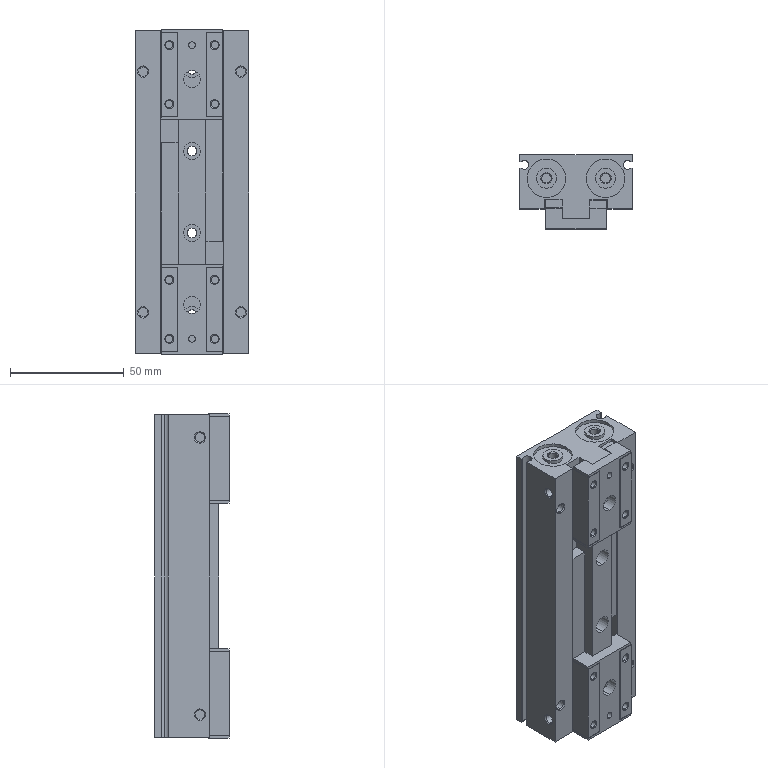Part | SolidWorks | 3 solids | 260 faces | box 50 x 33 x 142.8 mm | volume 178016 mm3 | plane 128 | cylinder 88 | cone 44 | commonest cylinder face diameters 4.134 x28 3.242 x16 7.5 x12 4 x8 4.3 x8 17 x8